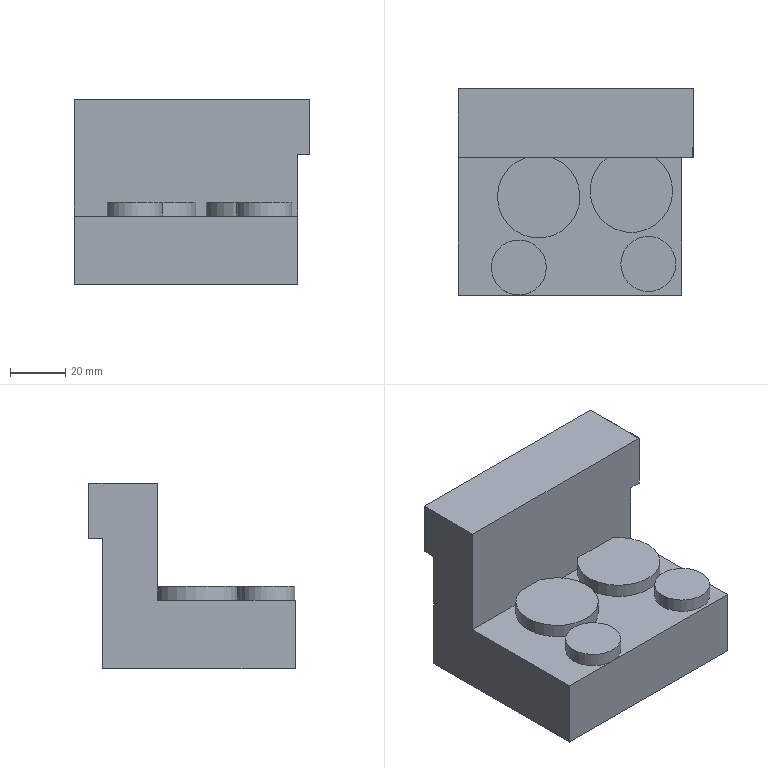Part | NX | features solid 2 | 1 solid | 21 faces | box 85.559 x 74.968 x 67.5 mm | volume 231490 mm3 | plane 14 | cylinder 4 | spline 3 | commonest cylinder face diameters 20 x2 30 x2
STEP:
#1=CARTESIAN_POINT('',(-954.807,-200.032,-82.5));
#2=VERTEX_POINT('',#1);
#3=CARTESIAN_POINT('',(-1040.,-200.032,-82.5));
#4=VERTEX_POINT('',#3);
#5=CARTESIAN_POINT('',(-954.807,-200.032,-82.5));
#6=CARTESIAN_POINT('',(-983.205,-200.032,-82.5));
#7=CARTESIAN_POINT('',(-1011.602,-200.032,-82.5));
#8=CARTESIAN_POINT('',(-1040.,-200.032,-82.5));
#9=B_SPLINE_CURVE_WITH_KNOTS('',3,(#5,#6,#7,#8),.UNSPECIFIED.,.F.,.F.,(4,4),(0.,0.08519),.UNSPECIFIED.);
#10=EDGE_CURVE('',#2,#4,#9,.T.);
#11=ORIENTED_EDGE('',*,*,#10,.T.);
#12=CARTESIAN_POINT('',(-1040.,-200.032,-125.));
#13=VERTEX_POINT('',#12);
#14=CARTESIAN_POINT('',(-1040.,-200.032,-77.5));
#15=DIRECTION('',(0.,0.,-1.));
#16=VECTOR('',#15,1000.);
#17=LINE('',#14,#16);
#18=EDGE_CURVE('',#4,#13,#17,.T.);
#19=ORIENTED_EDGE('',*,*,#18,.T.);
#20=CARTESIAN_POINT('',(-1015.637,-200.032,-125.));
#21=VERTEX_POINT('',#20);
#22=CARTESIAN_POINT('',(17.,-200.032,-125.));
#23=DIRECTION('',(-1.,0.,0.));
#24=VECTOR('',#23,1000.);
#25=LINE('',#22,#24);
#26=EDGE_CURVE('',#21,#13,#25,.T.);
#27=ORIENTED_EDGE('',*,*,#26,.F.);
#28=CARTESIAN_POINT('',(-1015.637,-200.032,-120.));
#29=VERTEX_POINT('',#28);
#30=CARTESIAN_POINT('',(-1015.637,-200.032,-122.5));
#31=DIRECTION('',(0.,0.,1.));
#32=VECTOR('',#31,1000.);
#33=LINE('',#30,#32);
#34=EDGE_CURVE('',#29,#21,#33,.F.);
#35=ORIENTED_EDGE('',*,*,#34,.F.);
#36=CARTESIAN_POINT('',(-1005.933,-200.032,-120.));
#37=VERTEX_POINT('',#36);
#38=CARTESIAN_POINT('',(-1010.785,-200.032,-120.));
#39=DIRECTION('',(-1.,0.,0.));
#40=VECTOR('',#39,1000.);
#41=LINE('',#38,#40);
#42=EDGE_CURVE('',#37,#29,#41,.T.);
#43=ORIENTED_EDGE('',*,*,#42,.F.);
#44=CARTESIAN_POINT('',(-1005.933,-200.032,-125.));
#45=VERTEX_POINT('',#44);
#46=CARTESIAN_POINT('',(-1005.933,-200.032,-122.5));
#47=DIRECTION('',(0.,0.,1.));
#48=VECTOR('',#47,1000.);
#49=LINE('',#46,#48);
#50=EDGE_CURVE('',#45,#37,#49,.T.);
#51=ORIENTED_EDGE('',*,*,#50,.F.);
#52=CARTESIAN_POINT('',(-985.912,-200.032,-125.));
#53=VERTEX_POINT('',#52);
#54=CARTESIAN_POINT('',(17.,-200.032,-125.));
#55=DIRECTION('',(-1.,0.,0.));
#56=VECTOR('',#55,1000.);
#57=LINE('',#54,#56);
#58=EDGE_CURVE('',#53,#45,#57,.T.);
#59=ORIENTED_EDGE('',*,*,#58,.F.);
#60=CARTESIAN_POINT('',(-985.912,-200.032,-120.));
#61=VERTEX_POINT('',#60);
#62=CARTESIAN_POINT('',(-985.912,-200.032,-122.5));
#63=DIRECTION('',(0.,0.,1.));
#64=VECTOR('',#63,1000.);
#65=LINE('',#62,#64);
#66=EDGE_CURVE('',#61,#53,#65,.F.);
#67=ORIENTED_EDGE('',*,*,#66,.F.);
#68=CARTESIAN_POINT('',(-968.282,-200.032,-120.));
#69=VERTEX_POINT('',#68);
#70=CARTESIAN_POINT('',(-977.097,-200.032,-120.));
#71=DIRECTION('',(-1.,0.,0.));
#72=VECTOR('',#71,1000.);
#73=LINE('',#70,#72);
#74=EDGE_CURVE('',#69,#61,#73,.T.);
#75=ORIENTED_EDGE('',*,*,#74,.F.);
#76=CARTESIAN_POINT('',(-968.282,-200.032,-125.));
#77=VERTEX_POINT('',#76);
#78=CARTESIAN_POINT('',(-968.282,-200.032,-122.5));
#79=DIRECTION('',(0.,0.,1.));
#80=VECTOR('',#79,1000.);
#81=LINE('',#78,#80);
#82=EDGE_CURVE('',#77,#69,#81,.T.);
#83=ORIENTED_EDGE('',*,*,#82,.F.);
#84=CARTESIAN_POINT('',(-958.74,-200.032,-125.));
#85=VERTEX_POINT('',#84);
#86=CARTESIAN_POINT('',(17.,-200.032,-125.));
#87=DIRECTION('',(-1.,0.,0.));
#88=VECTOR('',#87,1000.);
#89=LINE('',#86,#88);
#90=EDGE_CURVE('',#85,#77,#89,.T.);
#91=ORIENTED_EDGE('',*,*,#90,.F.);
#92=CARTESIAN_POINT('',(-958.74,-200.032,-102.5));
#93=VERTEX_POINT('',#92);
#94=CARTESIAN_POINT('',(-958.74,-200.032,-113.75));
#95=DIRECTION('',(0.,0.,-1.));
#96=VECTOR('',#95,1000.);
#97=LINE('',#94,#96);
#98=EDGE_CURVE('',#85,#93,#97,.F.);
#99=ORIENTED_EDGE('',*,*,#98,.T.);
#100=CARTESIAN_POINT('',(-954.807,-200.032,-102.5));
#101=VERTEX_POINT('',#100);
#102=CARTESIAN_POINT('',(-958.74,-200.032,-102.5));
#103=CARTESIAN_POINT('',(-957.429,-200.032,-102.5));
#104=CARTESIAN_POINT('',(-956.118,-200.032,-102.5));
#105=CARTESIAN_POINT('',(-954.807,-200.032,-102.5));
#106=B_SPLINE_CURVE_WITH_KNOTS('',3,(#102,#103,#104,#105),.UNSPECIFIED.,.F.,.F.,(4,4),(0.,0.003933),.UNSPECIFIED.);
#107=EDGE_CURVE('',#93,#101,#106,.T.);
#108=ORIENTED_EDGE('',*,*,#107,.T.);
#109=CARTESIAN_POINT('',(-954.441,-200.032,-102.5));
#110=VERTEX_POINT('',#109);
#111=CARTESIAN_POINT('',(-948.753,-200.032,-102.5));
#112=CARTESIAN_POINT('',(-953.753,-200.032,-102.5));
#113=CARTESIAN_POINT('',(-1031.831,-200.032,-102.5));
#114=CARTESIAN_POINT('',(-1036.831,-200.032,-102.5));
#115=CARTESIAN_POINT('',(-1037.712,-200.032,-102.5));
#116=B_SPLINE_CURVE_WITH_KNOTS('',1,(#111,#112,#113,#114,#115),.UNSPECIFIED.,.F.,.F.,(2,1,1,1,2),(-0.06404,0.,1.,1.064,1.075),.PIECEWISE_BEZIER_KNOTS.);
#117=EDGE_CURVE('',#110,#101,#116,.T.);
#118=ORIENTED_EDGE('',*,*,#117,.F.);
#119=CARTESIAN_POINT('',(-954.441,-200.032,-82.5));
#120=VERTEX_POINT('',#119);
#121=CARTESIAN_POINT('',(-954.441,-200.032,-92.5));
#122=DIRECTION('',(0.,0.,-1.));
#123=VECTOR('',#122,1000.);
#124=LINE('',#121,#123);
#125=EDGE_CURVE('',#120,#110,#124,.T.);
#126=ORIENTED_EDGE('',*,*,#125,.F.);
#127=CARTESIAN_POINT('',(-115.539,-200.032,-82.5));
#128=DIRECTION('',(-1.,0.,0.));
#129=VECTOR('',#128,1000.);
#130=LINE('',#127,#129);
#131=EDGE_CURVE('',#120,#2,#130,.T.);
#132=ORIENTED_EDGE('',*,*,#131,.T.);
#133=EDGE_LOOP('',(#11,#19,#27,#35,#43,#51,#59,#67,#75,#83,#91,#99,#108,#118,#126,#132));
#134=FACE_BOUND('',#133,.T.);
#135=CARTESIAN_POINT('',(-954.807,-200.032,-77.5));
#136=DIRECTION('',(0.,-1.,0.));
#137=DIRECTION('',(-1.,0.,0.));
#138=AXIS2_PLACEMENT_3D('',#135,#136,#137);
#139=PLANE('',#138);
#140=ADVANCED_FACE('',(#134),#139,.T.);
#141=CARTESIAN_POINT('',(-1040.,-180.032,-150.));
#142=VERTEX_POINT('',#141);
#143=CARTESIAN_POINT('',(-1040.,-250.,-150.));
#144=VERTEX_POINT('',#143);
#145=CARTESIAN_POINT('',(-1040.,110.,-150.));
#146=DIRECTION('',(0.,-1.,0.));
#147=VECTOR('',#146,1000.);
#148=LINE('',#145,#147);
#149=EDGE_CURVE('',#142,#144,#148,.T.);
#150=ORIENTED_EDGE('',*,*,#149,.F.);
#151=CARTESIAN_POINT('',(-958.75,-180.032,-150.));
#152=VERTEX_POINT('',#151);
#153=CARTESIAN_POINT('',(17.,-180.032,-150.));
#154=DIRECTION('',(-1.,0.,0.));
#155=VECTOR('',#154,1000.);
#156=LINE('',#153,#155);
#157=EDGE_CURVE('',#142,#152,#156,.F.);
#158=ORIENTED_EDGE('',*,*,#157,.T.);
#159=CARTESIAN_POINT('',(-958.747,-250.,-150.));
#160=VERTEX_POINT('',#159);
#161=CARTESIAN_POINT('',(-958.747,-250.,-150.));
#162=CARTESIAN_POINT('',(-958.747,-226.677,-150.));
#163=CARTESIAN_POINT('',(-958.747,-203.355,-150.));
#164=CARTESIAN_POINT('',(-958.747,-180.032,-150.));
#165=B_SPLINE_CURVE_WITH_KNOTS('',3,(#161,#162,#163,#164),.UNSPECIFIED.,.F.,.F.,(4,4),(0.07143,1.071),.UNSPECIFIED.);
#166=EDGE_CURVE('',#160,#152,#165,.T.);
#167=ORIENTED_EDGE('',*,*,#166,.F.);
#168=CARTESIAN_POINT('',(-953.753,-250.,-150.));
#169=DIRECTION('',(1.,0.,0.));
#170=VECTOR('',#169,1000.);
#171=LINE('',#168,#170);
#172=EDGE_CURVE('',#160,#144,#171,.F.);
#173=ORIENTED_EDGE('',*,*,#172,.T.);
#174=EDGE_LOOP('',(#150,#158,#167,#173));
#175=FACE_BOUND('',#174,.T.);
#176=CARTESIAN_POINT('',(17.,110.,-150.));
#177=DIRECTION('',(0.,0.,1.));
#178=DIRECTION('',(1.,0.,0.));
#179=AXIS2_PLACEMENT_3D('',#176,#177,#178);
#180=PLANE('',#179);
#181=ADVANCED_FACE('',(#175),#180,.F.);
#182=CARTESIAN_POINT('',(-954.441,-175.032,-82.5));
#183=VERTEX_POINT('',#182);
#184=CARTESIAN_POINT('',(-1040.,-175.032,-82.5));
#185=VERTEX_POINT('',#184);
#186=CARTESIAN_POINT('',(-115.539,-175.032,-82.5));
#187=DIRECTION('',(-1.,0.,0.));
#188=VECTOR('',#187,1000.);
#189=LINE('',#186,#188);
#190=EDGE_CURVE('',#183,#185,#189,.T.);
#191=ORIENTED_EDGE('',*,*,#190,.T.);
#192=CARTESIAN_POINT('',(-1040.,110.,-82.5));
#193=DIRECTION('',(0.,1.,0.));
#194=VECTOR('',#193,1000.);
#195=LINE('',#192,#194);
#196=EDGE_CURVE('',#185,#4,#195,.F.);
#197=ORIENTED_EDGE('',*,*,#196,.T.);
#198=ORIENTED_EDGE('',*,*,#10,.F.);
#199=CARTESIAN_POINT('',(-954.441,-175.032,-82.5));
#200=CARTESIAN_POINT('',(-954.452,-177.116,-82.5));
#201=CARTESIAN_POINT('',(-954.492,-181.283,-82.5));
#202=CARTESIAN_POINT('',(-954.384,-187.536,-82.5));
#203=CARTESIAN_POINT('',(-954.719,-193.782,-82.5));
#204=CARTESIAN_POINT('',(-954.794,-197.948,-82.5));
#205=CARTESIAN_POINT('',(-954.807,-200.032,-82.5));
#206=B_SPLINE_CURVE_WITH_KNOTS('',3,(#199,#200,#201,#202,#203,#204,#205),.UNSPECIFIED.,.F.,.F.,(4,1,1,1,4),(-0.004968,0.001283,0.007534,0.01378,0.02003),.UNSPECIFIED.);
#207=EDGE_CURVE('',#183,#2,#206,.T.);
#208=ORIENTED_EDGE('',*,*,#207,.F.);
#209=EDGE_LOOP('',(#191,#197,#198,#208));
#210=FACE_BOUND('',#209,.T.);
#211=CARTESIAN_POINT('',(-1040.,-175.032,-82.5));
#212=CARTESIAN_POINT('',(-1040.,-200.032,-82.5));
#213=CARTESIAN_POINT('',(-953.928,-175.032,-82.5));
#214=CARTESIAN_POINT('',(-953.928,-200.032,-82.5));
#215=B_SPLINE_SURFACE_WITH_KNOTS('',1,1,((#211,#212),(#213,#214)),.PLANE_SURF.,.F.,.F.,.F.,(2,2),(2,2),(0.1201,0.1555),(0.6584,0.6722),.PIECEWISE_BEZIER_KNOTS.);
#216=ADVANCED_FACE('',(#210),#215,.F.);
#217=CARTESIAN_POINT('',(-1040.,-250.,-125.));
#218=VERTEX_POINT('',#217);
#219=CARTESIAN_POINT('',(-1040.,-250.,-142.494));
#220=DIRECTION('',(0.,0.,-1.));
#221=VECTOR('',#220,1000.);
#222=LINE('',#219,#221);
#223=EDGE_CURVE('',#144,#218,#222,.F.);
#224=ORIENTED_EDGE('',*,*,#223,.F.);
#225=ORIENTED_EDGE('',*,*,#172,.F.);
#226=CARTESIAN_POINT('',(-958.746,-250.,-125.));
#227=VERTEX_POINT('',#226);
#228=CARTESIAN_POINT('',(-958.747,-250.,-125.));
#229=CARTESIAN_POINT('',(-958.747,-250.,-133.333));
#230=CARTESIAN_POINT('',(-958.747,-250.,-141.667));
#231=CARTESIAN_POINT('',(-958.747,-250.,-150.));
#232=B_SPLINE_CURVE_WITH_KNOTS('',3,(#228,#229,#230,#231),.UNSPECIFIED.,.F.,.F.,(4,4),(0.,1.),.UNSPECIFIED.);
#233=EDGE_CURVE('',#227,#160,#232,.T.);
#234=ORIENTED_EDGE('',*,*,#233,.F.);
#235=CARTESIAN_POINT('',(-953.753,-250.,-125.));
#236=DIRECTION('',(1.,0.,0.));
#237=VECTOR('',#236,1000.);
#238=LINE('',#235,#237);
#239=EDGE_CURVE('',#227,#218,#238,.F.);
#240=ORIENTED_EDGE('',*,*,#239,.T.);
#241=EDGE_LOOP('',(#224,#225,#234,#240));
#242=FACE_BOUND('',#241,.T.);
#243=CARTESIAN_POINT('',(-953.753,-250.,-142.494));
#244=DIRECTION('',(0.,-1.,0.));
#245=DIRECTION('',(-0.9998,0.,-0.01745));
#246=AXIS2_PLACEMENT_3D('',#243,#244,#245);
#247=PLANE('',#246);
#248=ADVANCED_FACE('',(#242),#247,.T.);
#249=CARTESIAN_POINT('',(-960.925,-238.656,-125.));
#250=VERTEX_POINT('',#249);
#251=CARTESIAN_POINT('',(-970.925,-238.656,-125.));
#252=DIRECTION('',(0.,0.,-1.));
#253=DIRECTION('',(1.,0.,0.));
#254=AXIS2_PLACEMENT_3D('',#251,#252,#253);
#255=CIRCLE('',#254,10.);
#256=EDGE_CURVE('',#250,#250,#255,.T.);
#257=ORIENTED_EDGE('',*,*,#256,.T.);
#258=EDGE_LOOP('',(#257));
#259=FACE_BOUND('',#258,.T.);
#260=CARTESIAN_POINT('',(-1007.986,-239.942,-125.));
#261=VERTEX_POINT('',#260);
#262=CARTESIAN_POINT('',(-1017.986,-239.942,-125.));
#263=DIRECTION('',(0.,0.,-1.));
#264=DIRECTION('',(1.,0.,0.));
#265=AXIS2_PLACEMENT_3D('',#262,#263,#264);
#266=CIRCLE('',#265,10.);
#267=EDGE_CURVE('',#261,#261,#266,.T.);
#268=ORIENTED_EDGE('',*,*,#267,.T.);
#269=EDGE_LOOP('',(#268));
#270=FACE_BOUND('',#269,.T.);
#271=ORIENTED_EDGE('',*,*,#26,.T.);
#272=CARTESIAN_POINT('',(-1040.,110.,-125.));
#273=DIRECTION('',(0.,-1.,0.));
#274=VECTOR('',#273,1000.);
#275=LINE('',#272,#274);
#276=EDGE_CURVE('',#13,#218,#275,.T.);
#277=ORIENTED_EDGE('',*,*,#276,.T.);
#278=ORIENTED_EDGE('',*,*,#239,.F.);
#279=CARTESIAN_POINT('',(-958.746,-250.,-125.));
#280=CARTESIAN_POINT('',(-958.744,-233.344,-125.));
#281=CARTESIAN_POINT('',(-958.739,-216.688,-125.));
#282=CARTESIAN_POINT('',(-958.74,-200.032,-125.));
#283=B_SPLINE_CURVE_WITH_KNOTS('',3,(#279,#280,#281,#282),.UNSPECIFIED.,.F.,.F.,(4,4),(-0.01,0.03997),.UNSPECIFIED.);
#284=EDGE_CURVE('',#227,#85,#283,.T.);
#285=ORIENTED_EDGE('',*,*,#284,.T.);
#286=ORIENTED_EDGE('',*,*,#90,.T.);
#287=CARTESIAN_POINT('',(-977.097,-212.168,-125.));
#288=DIRECTION('',(0.,0.,-1.));
#289=DIRECTION('',(1.,0.,0.));
#290=AXIS2_PLACEMENT_3D('',#287,#288,#289);
#291=CIRCLE('',#290,15.);
#292=EDGE_CURVE('',#77,#53,#291,.T.);
#293=ORIENTED_EDGE('',*,*,#292,.T.);
#294=ORIENTED_EDGE('',*,*,#58,.T.);
#295=CARTESIAN_POINT('',(-1010.785,-214.226,-125.));
#296=DIRECTION('',(0.,0.,-1.));
#297=DIRECTION('',(1.,0.,0.));
#298=AXIS2_PLACEMENT_3D('',#295,#296,#297);
#299=CIRCLE('',#298,15.);
#300=EDGE_CURVE('',#45,#21,#299,.T.);
#301=ORIENTED_EDGE('',*,*,#300,.T.);
#302=EDGE_LOOP('',(#271,#277,#278,#285,#286,#293,#294,#301));
#303=FACE_BOUND('',#302,.T.);
#304=CARTESIAN_POINT('',(17.,110.,-125.));
#305=DIRECTION('',(0.,0.,1.));
#306=DIRECTION('',(1.,0.,0.));
#307=AXIS2_PLACEMENT_3D('',#304,#305,#306);
#308=PLANE('',#307);
#309=ADVANCED_FACE('',(#259,#270,#303),#308,.T.);
#310=CARTESIAN_POINT('',(-1040.,-175.032,-102.5));
#311=VERTEX_POINT('',#310);
#312=CARTESIAN_POINT('',(-1040.,-180.032,-102.5));
#313=VERTEX_POINT('',#312);
#314=CARTESIAN_POINT('',(-1040.,-175.032,-102.5));
#315=DIRECTION('',(0.,-1.,0.));
#316=VECTOR('',#315,1000.);
#317=LINE('',#314,#316);
#318=EDGE_CURVE('',#311,#313,#317,.T.);
#319=ORIENTED_EDGE('',*,*,#318,.F.);
#320=CARTESIAN_POINT('',(-954.807,-175.032,-102.5));
#321=VERTEX_POINT('',#320);
#322=CARTESIAN_POINT('',(-1040.,-175.032,-102.5));
#323=CARTESIAN_POINT('',(-1011.602,-175.032,-102.5));
#324=CARTESIAN_POINT('',(-983.205,-175.032,-102.5));
#325=CARTESIAN_POINT('',(-954.807,-175.032,-102.5));
#326=B_SPLINE_CURVE_WITH_KNOTS('',3,(#322,#323,#324,#325),.UNSPECIFIED.,.F.,.F.,(4,4),(0.3305,0.4157),.UNSPECIFIED.);
#327=EDGE_CURVE('',#321,#311,#326,.F.);
#328=ORIENTED_EDGE('',*,*,#327,.F.);
#329=CARTESIAN_POINT('',(-954.807,-200.032,-102.5));
#330=DIRECTION('',(0.,-1.,0.));
#331=VECTOR('',#330,1000.);
#332=LINE('',#329,#331);
#333=EDGE_CURVE('',#101,#321,#332,.F.);
#334=ORIENTED_EDGE('',*,*,#333,.F.);
#335=ORIENTED_EDGE('',*,*,#107,.F.);
#336=CARTESIAN_POINT('',(-958.753,-180.032,-102.5));
#337=VERTEX_POINT('',#336);
#338=CARTESIAN_POINT('',(-958.753,-180.032,-102.5));
#339=CARTESIAN_POINT('',(-958.744,-186.699,-102.5));
#340=CARTESIAN_POINT('',(-958.74,-193.365,-102.5));
#341=CARTESIAN_POINT('',(-958.74,-200.032,-102.5));
#342=B_SPLINE_CURVE_WITH_KNOTS('',3,(#338,#339,#340,#341),.UNSPECIFIED.,.F.,.F.,(4,4),(0.1419,0.1619),.UNSPECIFIED.);
#343=EDGE_CURVE('',#337,#93,#342,.T.);
#344=ORIENTED_EDGE('',*,*,#343,.F.);
#345=CARTESIAN_POINT('',(-1011.957,-180.032,-102.5));
#346=VERTEX_POINT('',#345);
#347=CARTESIAN_POINT('',(-954.441,-180.032,-102.5));
#348=CARTESIAN_POINT('',(-1031.831,-180.032,-102.5));
#349=CARTESIAN_POINT('',(-1036.831,-180.032,-102.5));
#350=CARTESIAN_POINT('',(-1037.653,-180.032,-102.5));
#351=B_SPLINE_CURVE_WITH_KNOTS('',1,(#347,#348,#349,#350),.UNSPECIFIED.,.F.,.F.,(2,1,1,2),(0.,0.93,0.9901,1.),.UNSPECIFIED.);
#352=EDGE_CURVE('',#337,#346,#351,.T.);
#353=ORIENTED_EDGE('',*,*,#352,.T.);
#354=CARTESIAN_POINT('',(-1011.957,-180.032,-102.5));
#355=CARTESIAN_POINT('',(-1021.305,-180.032,-102.5));
#356=CARTESIAN_POINT('',(-1030.652,-180.032,-102.5));
#357=CARTESIAN_POINT('',(-1040.,-180.032,-102.5));
#358=B_SPLINE_CURVE_WITH_KNOTS('',3,(#354,#355,#356,#357),.UNSPECIFIED.,.F.,.F.,(4,4),(0.,0.02804),.UNSPECIFIED.);
#359=EDGE_CURVE('',#346,#313,#358,.T.);
#360=ORIENTED_EDGE('',*,*,#359,.T.);
#361=EDGE_LOOP('',(#319,#328,#334,#335,#344,#353,#360));
#362=FACE_BOUND('',#361,.T.);
#363=CARTESIAN_POINT('',(-954.807,-175.032,-102.5));
#364=CARTESIAN_POINT('',(-954.807,-200.032,-102.5));
#365=CARTESIAN_POINT('',(-1031.831,-175.032,-102.5));
#366=CARTESIAN_POINT('',(-1031.831,-200.032,-102.5));
#367=CARTESIAN_POINT('',(-1036.831,-175.032,-102.5));
#368=CARTESIAN_POINT('',(-1036.831,-200.032,-102.5));
#369=CARTESIAN_POINT('',(-1037.653,-175.032,-102.5));
#370=CARTESIAN_POINT('',(-1037.653,-200.032,-102.5));
#371=CARTESIAN_POINT('',(-1040.,-175.032,-102.5));
#372=CARTESIAN_POINT('',(-1040.,-200.032,-102.5));
#373=B_SPLINE_SURFACE_WITH_KNOTS('',1,1,((#363,#364),(#365,#366),(#367,#368),(#369,#370),(#371,#372)),.SURF_OF_LINEAR_EXTRUSION.,.F.,.F.,.F.,(2,1,1,1,2),(2,2),(0.004399,0.93,0.9901,1.,1.028),(0.,1.),.PIECEWISE_BEZIER_KNOTS.);
#374=ADVANCED_FACE('',(#362),#373,.F.);
#375=CARTESIAN_POINT('',(-1040.,-175.032,-77.5));
#376=DIRECTION('',(0.,0.,-1.));
#377=VECTOR('',#376,1000.);
#378=LINE('',#375,#377);
#379=EDGE_CURVE('',#185,#311,#378,.T.);
#380=ORIENTED_EDGE('',*,*,#379,.F.);
#381=ORIENTED_EDGE('',*,*,#190,.F.);
#382=CARTESIAN_POINT('',(-954.441,-175.032,-102.5));
#383=VERTEX_POINT('',#382);
#384=CARTESIAN_POINT('',(-954.441,-175.032,-92.5));
#385=DIRECTION('',(0.,0.,-1.));
#386=VECTOR('',#385,1000.);
#387=LINE('',#384,#386);
#388=EDGE_CURVE('',#183,#383,#387,.T.);
#389=ORIENTED_EDGE('',*,*,#388,.T.);
#390=CARTESIAN_POINT('',(-954.807,-175.032,-102.5));
#391=DIRECTION('',(-1.,0.,0.));
#392=VECTOR('',#391,1000.);
#393=LINE('',#390,#392);
#394=EDGE_CURVE('',#383,#321,#393,.T.);
#395=ORIENTED_EDGE('',*,*,#394,.T.);
#396=ORIENTED_EDGE('',*,*,#327,.T.);
#397=EDGE_LOOP('',(#380,#381,#389,#395,#396));
#398=FACE_BOUND('',#397,.T.);
#399=CARTESIAN_POINT('',(-954.807,-175.032,-77.5));
#400=DIRECTION('',(0.,-1.,0.));
#401=DIRECTION('',(-1.,0.,0.));
#402=AXIS2_PLACEMENT_3D('',#399,#400,#401);
#403=PLANE('',#402);
#404=ADVANCED_FACE('',(#398),#403,.F.);
#405=CARTESIAN_POINT('',(-1040.,-180.032,-302.5));
#406=DIRECTION('',(0.,0.,-1.));
#407=VECTOR('',#406,1000.);
#408=LINE('',#405,#407);
#409=EDGE_CURVE('',#313,#142,#408,.T.);
#410=ORIENTED_EDGE('',*,*,#409,.F.);
#411=ORIENTED_EDGE('',*,*,#359,.F.);
#412=ORIENTED_EDGE('',*,*,#352,.F.);
#413=CARTESIAN_POINT('',(-958.753,-180.032,-126.25));
#414=DIRECTION('',(0.,0.,-1.));
#415=VECTOR('',#414,1000.);
#416=LINE('',#413,#415);
#417=EDGE_CURVE('',#337,#152,#416,.T.);
#418=ORIENTED_EDGE('',*,*,#417,.T.);
#419=ORIENTED_EDGE('',*,*,#157,.F.);
#420=EDGE_LOOP('',(#410,#411,#412,#418,#419));
#421=FACE_BOUND('',#420,.T.);
#422=CARTESIAN_POINT('',(-954.441,-180.032,-302.5));
#423=DIRECTION('',(0.,-1.,0.));
#424=DIRECTION('',(-1.,0.,0.));
#425=AXIS2_PLACEMENT_3D('',#422,#423,#424);
#426=PLANE('',#425);
#427=ADVANCED_FACE('',(#421),#426,.F.);
#428=ORIENTED_EDGE('',*,*,#343,.T.);
#429=ORIENTED_EDGE('',*,*,#98,.F.);
#430=ORIENTED_EDGE('',*,*,#284,.F.);
#431=ORIENTED_EDGE('',*,*,#233,.T.);
#432=ORIENTED_EDGE('',*,*,#166,.T.);
#433=ORIENTED_EDGE('',*,*,#417,.F.);
#434=EDGE_LOOP('',(#428,#429,#430,#431,#432,#433));
#435=FACE_BOUND('',#434,.T.);
#436=CARTESIAN_POINT('',(-958.753,-180.032,-102.5));
#437=CARTESIAN_POINT('',(-958.753,-180.032,-150.));
#438=CARTESIAN_POINT('',(-958.721,-203.347,-102.5));
#439=CARTESIAN_POINT('',(-958.721,-203.347,-150.));
#440=CARTESIAN_POINT('',(-958.743,-226.675,-102.5));
#441=CARTESIAN_POINT('',(-958.743,-226.675,-150.));
#442=CARTESIAN_POINT('',(-958.746,-250.,-102.5));
#443=CARTESIAN_POINT('',(-958.746,-250.,-150.));
#444=B_SPLINE_SURFACE_WITH_KNOTS('',3,1,((#436,#437),(#438,#439),(#440,#441),(#442,#443)),.SURF_OF_LINEAR_EXTRUSION.,.F.,.F.,.F.,(4,4),(2,2),(0.001006,2.8),(0.,1.),.PIECEWISE_BEZIER_KNOTS.);
#445=ADVANCED_FACE('',(#435),#444,.T.);
#446=ORIENTED_EDGE('',*,*,#74,.T.);
#447=CARTESIAN_POINT('',(-977.097,-212.168,-120.));
#448=DIRECTION('',(0.,0.,-1.));
#449=DIRECTION('',(1.,0.,0.));
#450=AXIS2_PLACEMENT_3D('',#447,#448,#449);
#451=CIRCLE('',#450,15.);
#452=EDGE_CURVE('',#69,#61,#451,.T.);
#453=ORIENTED_EDGE('',*,*,#452,.F.);
#454=EDGE_LOOP('',(#446,#453));
#455=FACE_BOUND('',#454,.T.);
#456=CARTESIAN_POINT('',(-977.097,-217.168,-120.));
#457=DIRECTION('',(0.,0.,1.));
#458=DIRECTION('',(1.,0.,0.));
#459=AXIS2_PLACEMENT_3D('',#456,#457,#458);
#460=PLANE('',#459);
#461=ADVANCED_FACE('',(#455),#460,.T.);
#462=ORIENTED_EDGE('',*,*,#66,.T.);
#463=ORIENTED_EDGE('',*,*,#292,.F.);
#464=ORIENTED_EDGE('',*,*,#82,.T.);
#465=ORIENTED_EDGE('',*,*,#452,.T.);
#466=EDGE_LOOP('',(#462,#463,#464,#465));
#467=FACE_BOUND('',#466,.T.);
#468=CARTESIAN_POINT('',(-977.097,-212.168,-125.));
#469=DIRECTION('',(0.,0.,1.));
#470=DIRECTION('',(1.,0.,0.));
#471=AXIS2_PLACEMENT_3D('',#468,#469,#470);
#472=CYLINDRICAL_SURFACE('',#471,15.);
#473=ADVANCED_FACE('',(#467),#472,.T.);
#474=ORIENTED_EDGE('',*,*,#42,.T.);
#475=CARTESIAN_POINT('',(-1010.785,-214.226,-120.));
#476=DIRECTION('',(0.,0.,-1.));
#477=DIRECTION('',(1.,0.,0.));
#478=AXIS2_PLACEMENT_3D('',#475,#476,#477);
#479=CIRCLE('',#478,15.);
#480=EDGE_CURVE('',#37,#29,#479,.T.);
#481=ORIENTED_EDGE('',*,*,#480,.F.);
#482=EDGE_LOOP('',(#474,#481));
#483=FACE_BOUND('',#482,.T.);
#484=CARTESIAN_POINT('',(-1010.785,-219.226,-120.));
#485=DIRECTION('',(0.,0.,1.));
#486=DIRECTION('',(1.,0.,0.));
#487=AXIS2_PLACEMENT_3D('',#484,#485,#486);
#488=PLANE('',#487);
#489=ADVANCED_FACE('',(#483),#488,.T.);
#490=ORIENTED_EDGE('',*,*,#34,.T.);
#491=ORIENTED_EDGE('',*,*,#300,.F.);
#492=ORIENTED_EDGE('',*,*,#50,.T.);
#493=ORIENTED_EDGE('',*,*,#480,.T.);
#494=EDGE_LOOP('',(#490,#491,#492,#493));
#495=FACE_BOUND('',#494,.T.);
#496=CARTESIAN_POINT('',(-1010.785,-214.226,-125.));
#497=DIRECTION('',(0.,0.,1.));
#498=DIRECTION('',(1.,0.,0.));
#499=AXIS2_PLACEMENT_3D('',#496,#497,#498);
#500=CYLINDRICAL_SURFACE('',#499,15.);
#501=ADVANCED_FACE('',(#495),#500,.T.);
#502=CARTESIAN_POINT('',(-960.925,-238.656,-120.));
#503=VERTEX_POINT('',#502);
#504=CARTESIAN_POINT('',(-970.925,-238.656,-120.));
#505=DIRECTION('',(0.,0.,-1.));
#506=DIRECTION('',(1.,0.,0.));
#507=AXIS2_PLACEMENT_3D('',#504,#505,#506);
#508=CIRCLE('',#507,10.);
#509=EDGE_CURVE('',#503,#503,#508,.T.);
#510=ORIENTED_EDGE('',*,*,#509,.F.);
#511=EDGE_LOOP('',(#510));
#512=FACE_BOUND('',#511,.T.);
#513=CARTESIAN_POINT('',(-1010.785,-219.226,-120.));
#514=DIRECTION('',(0.,0.,1.));
#515=DIRECTION('',(1.,0.,0.));
#516=AXIS2_PLACEMENT_3D('',#513,#514,#515);
#517=PLANE('',#516);
#518=ADVANCED_FACE('',(#512),#517,.T.);
#519=ORIENTED_EDGE('',*,*,#509,.T.);
#520=EDGE_LOOP('',(#519));
#521=FACE_BOUND('',#520,.T.);
#522=ORIENTED_EDGE('',*,*,#256,.F.);
#523=EDGE_LOOP('',(#522));
#524=FACE_BOUND('',#523,.T.);
#525=CARTESIAN_POINT('',(-970.925,-238.656,-125.));
#526=DIRECTION('',(0.,0.,1.));
#527=DIRECTION('',(1.,0.,0.));
#528=AXIS2_PLACEMENT_3D('',#525,#526,#527);
#529=CYLINDRICAL_SURFACE('',#528,10.);
#530=ADVANCED_FACE('',(#521,#524),#529,.T.);
#531=CARTESIAN_POINT('',(-1007.986,-239.942,-120.));
#532=VERTEX_POINT('',#531);
#533=CARTESIAN_POINT('',(-1017.986,-239.942,-120.));
#534=DIRECTION('',(0.,0.,-1.));
#535=DIRECTION('',(1.,0.,0.));
#536=AXIS2_PLACEMENT_3D('',#533,#534,#535);
#537=CIRCLE('',#536,10.);
#538=EDGE_CURVE('',#532,#532,#537,.T.);
#539=ORIENTED_EDGE('',*,*,#538,.F.);
#540=EDGE_LOOP('',(#539));
#541=FACE_BOUND('',#540,.T.);
#542=CARTESIAN_POINT('',(-1010.785,-219.226,-120.));
#543=DIRECTION('',(0.,0.,1.));
#544=DIRECTION('',(1.,0.,0.));
#545=AXIS2_PLACEMENT_3D('',#542,#543,#544);
#546=PLANE('',#545);
#547=ADVANCED_FACE('',(#541),#546,.T.);
#548=ORIENTED_EDGE('',*,*,#538,.T.);
#549=EDGE_LOOP('',(#548));
#550=FACE_BOUND('',#549,.T.);
#551=ORIENTED_EDGE('',*,*,#267,.F.);
#552=EDGE_LOOP('',(#551));
#553=FACE_BOUND('',#552,.T.);
#554=CARTESIAN_POINT('',(-1017.986,-239.942,-125.));
#555=DIRECTION('',(0.,0.,1.));
#556=DIRECTION('',(1.,0.,0.));
#557=AXIS2_PLACEMENT_3D('',#554,#555,#556);
#558=CYLINDRICAL_SURFACE('',#557,10.);
#559=ADVANCED_FACE('',(#550,#553),#558,.T.);
#560=ORIENTED_EDGE('',*,*,#131,.F.);
#561=CARTESIAN_POINT('',(-954.441,-175.032,-82.5));
#562=DIRECTION('',(0.,-1.,0.));
#563=VECTOR('',#562,1000.);
#564=LINE('',#561,#563);
#565=EDGE_CURVE('',#183,#120,#564,.T.);
#566=ORIENTED_EDGE('',*,*,#565,.F.);
#567=ORIENTED_EDGE('',*,*,#207,.T.);
#568=EDGE_LOOP('',(#560,#566,#567));
#569=FACE_BOUND('',#568,.T.);
#570=CARTESIAN_POINT('',(-115.539,-175.032,-82.5));
#571=DIRECTION('',(0.,0.,-1.));
#572=DIRECTION('',(-1.,0.,0.));
#573=AXIS2_PLACEMENT_3D('',#570,#571,#572);
#574=PLANE('',#573);
#575=ADVANCED_FACE('',(#569),#574,.F.);
#576=ORIENTED_EDGE('',*,*,#117,.T.);
#577=ORIENTED_EDGE('',*,*,#333,.T.);
#578=ORIENTED_EDGE('',*,*,#394,.F.);
#579=CARTESIAN_POINT('',(-954.441,-175.032,-102.5));
#580=DIRECTION('',(0.,-1.,0.));
#581=VECTOR('',#580,1000.);
#582=LINE('',#579,#581);
#583=EDGE_CURVE('',#383,#110,#582,.T.);
#584=ORIENTED_EDGE('',*,*,#583,.T.);
#585=EDGE_LOOP('',(#576,#577,#578,#584));
#586=FACE_BOUND('',#585,.T.);
#587=CARTESIAN_POINT('',(-954.441,-175.032,-102.5));
#588=DIRECTION('',(0.,0.,-1.));
#589=DIRECTION('',(-1.,0.,0.));
#590=AXIS2_PLACEMENT_3D('',#587,#588,#589);
#591=PLANE('',#590);
#592=ADVANCED_FACE('',(#586),#591,.T.);
#593=ORIENTED_EDGE('',*,*,#125,.T.);
#594=ORIENTED_EDGE('',*,*,#583,.F.);
#595=ORIENTED_EDGE('',*,*,#388,.F.);
#596=ORIENTED_EDGE('',*,*,#565,.T.);
#597=EDGE_LOOP('',(#593,#594,#595,#596));
#598=FACE_BOUND('',#597,.T.);
#599=CARTESIAN_POINT('',(-954.441,-175.032,-92.5));
#600=DIRECTION('',(1.,0.,0.));
#601=DIRECTION('',(0.,0.,-1.));
#602=AXIS2_PLACEMENT_3D('',#599,#600,#601);
#603=PLANE('',#602);
#604=ADVANCED_FACE('',(#598),#603,.T.);
#605=ORIENTED_EDGE('',*,*,#276,.F.);
#606=ORIENTED_EDGE('',*,*,#18,.F.);
#607=ORIENTED_EDGE('',*,*,#196,.F.);
#608=ORIENTED_EDGE('',*,*,#379,.T.);
#609=ORIENTED_EDGE('',*,*,#318,.T.);
#610=ORIENTED_EDGE('',*,*,#409,.T.);
#611=ORIENTED_EDGE('',*,*,#149,.T.);
#612=ORIENTED_EDGE('',*,*,#223,.T.);
#613=EDGE_LOOP('',(#605,#606,#607,#608,#609,#610,#611,#612));
#614=FACE_BOUND('',#613,.T.);
#615=CARTESIAN_POINT('',(-1040.,-175.,0.));
#616=DIRECTION('',(-1.,0.,0.));
#617=DIRECTION('',(0.,0.,1.));
#618=AXIS2_PLACEMENT_3D('',#615,#616,#617);
#619=PLANE('',#618);
#620=ADVANCED_FACE('',(#614),#619,.T.);
#621=CLOSED_SHELL('',(#140,#181,#216,#248,#309,#374,#404,#427,#445,#461,#473,#489,#501,#518,#530,#547,#559,#575,#592,#604,#620));
#622=MANIFOLD_SOLID_BREP('',#621);
#623=(LENGTH_UNIT()NAMED_UNIT(*)SI_UNIT(.MILLI.,.METRE.));
#624=UNCERTAINTY_MEASURE_WITH_UNIT(LENGTH_MEASURE(0.05664),#623,'','');
#625=(NAMED_UNIT(*)PLANE_ANGLE_UNIT()SI_UNIT($,.RADIAN.));
#626=(NAMED_UNIT(*)SI_UNIT($,.STERADIAN.)SOLID_ANGLE_UNIT());
#627=(GEOMETRIC_REPRESENTATION_CONTEXT(3)GLOBAL_UNCERTAINTY_ASSIGNED_CONTEXT((#624))GLOBAL_UNIT_ASSIGNED_CONTEXT((#623,#625,#626))REPRESENTATION_CONTEXT('',''));
#628=ADVANCED_BREP_SHAPE_REPRESENTATION('',(#622),#627);